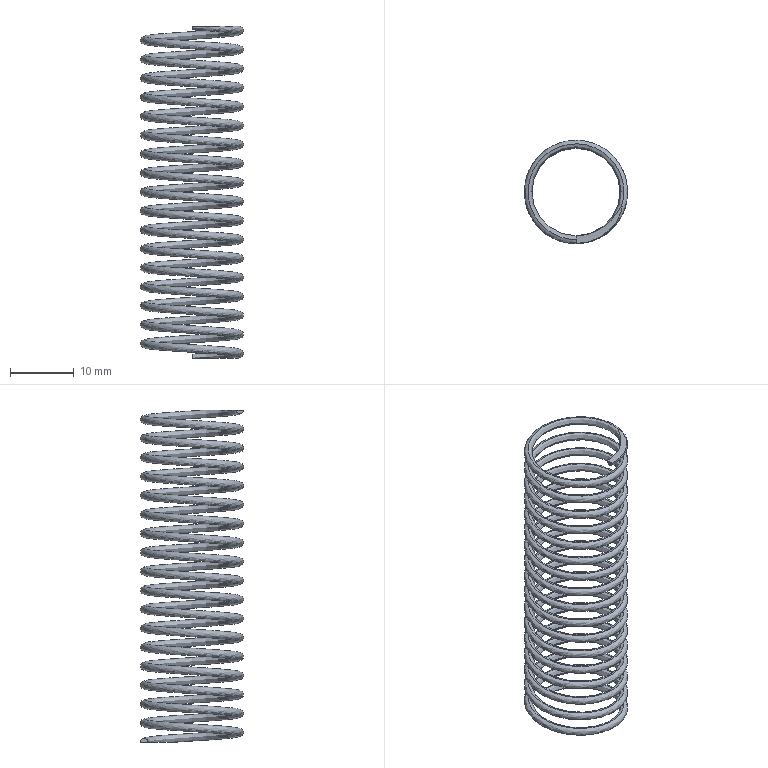Part | STEP file | Floating spring | 1 solid | 6 faces | box 16.2 x 16.2 x 52 mm | volume 929.653 mm3 | plane 4 | spline 2